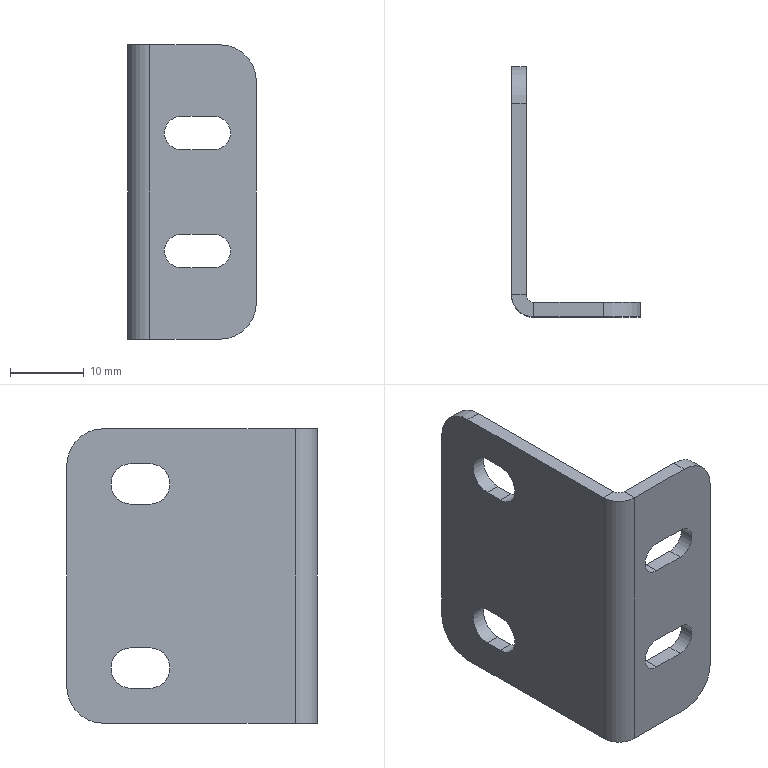Part | SolidWorks | features HoleWzd 2, Fillet 1, FlatPattern 1, SMBaseFlange 1, SheetMetal 1 | 1 solid | 34 faces | box 17.5 x 34 x 40 mm | volume 3554 mm3 | plane 20 | cylinder 14 | commonest cylinder face diameters 4.5 x4 5.5 x4 10 x4 2 x1 6 x1
STEP:
#1=CARTESIAN_POINT('',(0.,-31.,40.));
#2=VERTEX_POINT('',#1);
#3=CARTESIAN_POINT('',(2.,-31.,40.));
#4=VERTEX_POINT('',#3);
#5=CARTESIAN_POINT('',(0.,-31.,40.));
#6=DIRECTION('',(1.,0.,0.));
#7=VECTOR('',#6,1000.);
#8=LINE('',#5,#7);
#9=EDGE_CURVE('',#2,#4,#8,.T.);
#10=ORIENTED_EDGE('',*,*,#9,.F.);
#11=CARTESIAN_POINT('',(3.,-34.,40.));
#12=VERTEX_POINT('',#11);
#13=CARTESIAN_POINT('',(3.,-31.,40.));
#14=DIRECTION('',(0.,0.,1.));
#15=DIRECTION('',(-1.,0.,0.));
#16=AXIS2_PLACEMENT_3D('',#13,#14,#15);
#17=CIRCLE('',#16,3.);
#18=EDGE_CURVE('',#2,#12,#17,.T.);
#19=ORIENTED_EDGE('',*,*,#18,.T.);
#20=CARTESIAN_POINT('',(3.,-32.,40.));
#21=VERTEX_POINT('',#20);
#22=CARTESIAN_POINT('',(3.,-32.,40.));
#23=DIRECTION('',(0.,-1.,0.));
#24=VECTOR('',#23,1000.);
#25=LINE('',#22,#24);
#26=EDGE_CURVE('',#21,#12,#25,.T.);
#27=ORIENTED_EDGE('',*,*,#26,.F.);
#28=CARTESIAN_POINT('',(3.,-31.,40.));
#29=DIRECTION('',(0.,0.,1.));
#30=DIRECTION('',(1.,0.,0.));
#31=AXIS2_PLACEMENT_3D('',#28,#29,#30);
#32=CIRCLE('',#31,1.);
#33=EDGE_CURVE('',#4,#21,#32,.T.);
#34=ORIENTED_EDGE('',*,*,#33,.F.);
#35=EDGE_LOOP('',(#10,#19,#27,#34));
#36=FACE_OUTER_BOUND('',#35,.T.);
#37=CARTESIAN_POINT('',(0.,-31.,40.));
#38=DIRECTION('',(0.,0.,1.));
#39=DIRECTION('',(1.,0.,0.));
#40=AXIS2_PLACEMENT_3D('',#37,#38,#39);
#41=PLANE('',#40);
#42=ADVANCED_FACE('',(#36),#41,.T.);
#43=CARTESIAN_POINT('',(2.,-5.,40.));
#44=VERTEX_POINT('',#43);
#45=CARTESIAN_POINT('',(2.,0.,40.));
#46=DIRECTION('',(0.,-1.,0.));
#47=VECTOR('',#46,1000.);
#48=LINE('',#45,#47);
#49=EDGE_CURVE('',#44,#4,#48,.T.);
#50=ORIENTED_EDGE('',*,*,#49,.F.);
#51=CARTESIAN_POINT('',(0.,-5.,40.));
#52=VERTEX_POINT('',#51);
#53=CARTESIAN_POINT('',(3.,-5.,40.));
#54=DIRECTION('',(-1.,0.,0.));
#55=VECTOR('',#54,1000.);
#56=LINE('',#53,#55);
#57=EDGE_CURVE('',#44,#52,#56,.T.);
#58=ORIENTED_EDGE('',*,*,#57,.T.);
#59=CARTESIAN_POINT('',(0.,0.,40.));
#60=DIRECTION('',(0.,-1.,0.));
#61=VECTOR('',#60,1000.);
#62=LINE('',#59,#61);
#63=EDGE_CURVE('',#52,#2,#62,.T.);
#64=ORIENTED_EDGE('',*,*,#63,.T.);
#65=ORIENTED_EDGE('',*,*,#9,.T.);
#66=EDGE_LOOP('',(#50,#58,#64,#65));
#67=FACE_OUTER_BOUND('',#66,.T.);
#68=CARTESIAN_POINT('',(3.,-32.,40.));
#69=DIRECTION('',(0.,0.,1.));
#70=DIRECTION('',(1.,0.,0.));
#71=AXIS2_PLACEMENT_3D('',#68,#69,#70);
#72=PLANE('',#71);
#73=ADVANCED_FACE('',(#67),#72,.T.);
#74=CARTESIAN_POINT('',(3.,-34.,0.));
#75=VERTEX_POINT('',#74);
#76=CARTESIAN_POINT('',(3.,-32.,0.));
#77=VERTEX_POINT('',#76);
#78=CARTESIAN_POINT('',(3.,-34.,0.));
#79=DIRECTION('',(0.,1.,0.));
#80=VECTOR('',#79,1000.);
#81=LINE('',#78,#80);
#82=EDGE_CURVE('',#75,#77,#81,.T.);
#83=ORIENTED_EDGE('',*,*,#82,.F.);
#84=CARTESIAN_POINT('',(0.,-31.,0.));
#85=VERTEX_POINT('',#84);
#86=CARTESIAN_POINT('',(3.,-31.,0.));
#87=DIRECTION('',(0.,0.,1.));
#88=DIRECTION('',(-1.,0.,0.));
#89=AXIS2_PLACEMENT_3D('',#86,#87,#88);
#90=CIRCLE('',#89,3.);
#91=EDGE_CURVE('',#85,#75,#90,.T.);
#92=ORIENTED_EDGE('',*,*,#91,.F.);
#93=CARTESIAN_POINT('',(2.,-31.,0.));
#94=VERTEX_POINT('',#93);
#95=CARTESIAN_POINT('',(2.,-31.,0.));
#96=DIRECTION('',(-1.,0.,0.));
#97=VECTOR('',#96,1000.);
#98=LINE('',#95,#97);
#99=EDGE_CURVE('',#94,#85,#98,.T.);
#100=ORIENTED_EDGE('',*,*,#99,.F.);
#101=CARTESIAN_POINT('',(3.,-31.,0.));
#102=DIRECTION('',(0.,0.,1.));
#103=DIRECTION('',(1.,0.,0.));
#104=AXIS2_PLACEMENT_3D('',#101,#102,#103);
#105=CIRCLE('',#104,1.);
#106=EDGE_CURVE('',#94,#77,#105,.T.);
#107=ORIENTED_EDGE('',*,*,#106,.T.);
#108=EDGE_LOOP('',(#83,#92,#100,#107));
#109=FACE_OUTER_BOUND('',#108,.T.);
#110=CARTESIAN_POINT('',(3.,-34.,0.));
#111=DIRECTION('',(0.,0.,-1.));
#112=DIRECTION('',(-1.,0.,0.));
#113=AXIS2_PLACEMENT_3D('',#110,#111,#112);
#114=PLANE('',#113);
#115=ADVANCED_FACE('',(#109),#114,.T.);
#116=CARTESIAN_POINT('',(12.5,-32.,0.));
#117=VERTEX_POINT('',#116);
#118=CARTESIAN_POINT('',(0.,-32.,0.));
#119=DIRECTION('',(1.,0.,0.));
#120=VECTOR('',#119,1000.);
#121=LINE('',#118,#120);
#122=EDGE_CURVE('',#77,#117,#121,.T.);
#123=ORIENTED_EDGE('',*,*,#122,.T.);
#124=CARTESIAN_POINT('',(12.5,-34.,0.));
#125=VERTEX_POINT('',#124);
#126=CARTESIAN_POINT('',(12.5,-31.,0.));
#127=DIRECTION('',(0.,-1.,0.));
#128=VECTOR('',#127,1000.);
#129=LINE('',#126,#128);
#130=EDGE_CURVE('',#117,#125,#129,.T.);
#131=ORIENTED_EDGE('',*,*,#130,.T.);
#132=CARTESIAN_POINT('',(0.,-34.,0.));
#133=DIRECTION('',(1.,0.,0.));
#134=VECTOR('',#133,1000.);
#135=LINE('',#132,#134);
#136=EDGE_CURVE('',#75,#125,#135,.T.);
#137=ORIENTED_EDGE('',*,*,#136,.F.);
#138=ORIENTED_EDGE('',*,*,#82,.T.);
#139=EDGE_LOOP('',(#123,#131,#137,#138));
#140=FACE_OUTER_BOUND('',#139,.T.);
#141=CARTESIAN_POINT('',(2.,-31.,0.));
#142=DIRECTION('',(0.,0.,-1.));
#143=DIRECTION('',(-1.,0.,0.));
#144=AXIS2_PLACEMENT_3D('',#141,#142,#143);
#145=PLANE('',#144);
#146=ADVANCED_FACE('',(#140),#145,.T.);
#147=CARTESIAN_POINT('',(11.75,-34.,9.75));
#148=VERTEX_POINT('',#147);
#149=CARTESIAN_POINT('',(7.25,-34.,9.75));
#150=VERTEX_POINT('',#149);
#151=CARTESIAN_POINT('',(0.,-34.,9.75));
#152=DIRECTION('',(-1.,0.,0.));
#153=VECTOR('',#152,1000.);
#154=LINE('',#151,#153);
#155=EDGE_CURVE('',#148,#150,#154,.T.);
#156=ORIENTED_EDGE('',*,*,#155,.T.);
#157=CARTESIAN_POINT('',(7.25,-34.,14.25));
#158=VERTEX_POINT('',#157);
#159=CARTESIAN_POINT('',(7.25,-34.,12.));
#160=DIRECTION('',(0.,1.,0.));
#161=DIRECTION('',(0.,0.,1.));
#162=AXIS2_PLACEMENT_3D('',#159,#160,#161);
#163=CIRCLE('',#162,2.25);
#164=EDGE_CURVE('',#150,#158,#163,.T.);
#165=ORIENTED_EDGE('',*,*,#164,.T.);
#166=CARTESIAN_POINT('',(11.75,-34.,14.25));
#167=VERTEX_POINT('',#166);
#168=CARTESIAN_POINT('',(0.,-34.,14.25));
#169=DIRECTION('',(1.,0.,0.));
#170=VECTOR('',#169,1000.);
#171=LINE('',#168,#170);
#172=EDGE_CURVE('',#158,#167,#171,.T.);
#173=ORIENTED_EDGE('',*,*,#172,.T.);
#174=CARTESIAN_POINT('',(11.75,-34.,12.));
#175=DIRECTION('',(0.,1.,0.));
#176=DIRECTION('',(0.,0.,1.));
#177=AXIS2_PLACEMENT_3D('',#174,#175,#176);
#178=CIRCLE('',#177,2.25);
#179=EDGE_CURVE('',#167,#148,#178,.T.);
#180=ORIENTED_EDGE('',*,*,#179,.T.);
#181=EDGE_LOOP('',(#156,#165,#173,#180));
#182=FACE_BOUND('',#181,.T.);
#183=CARTESIAN_POINT('',(7.25,-34.,30.25));
#184=VERTEX_POINT('',#183);
#185=CARTESIAN_POINT('',(11.75,-34.,30.25));
#186=VERTEX_POINT('',#185);
#187=CARTESIAN_POINT('',(0.,-34.,30.25));
#188=DIRECTION('',(1.,0.,0.));
#189=VECTOR('',#188,1000.);
#190=LINE('',#187,#189);
#191=EDGE_CURVE('',#184,#186,#190,.T.);
#192=ORIENTED_EDGE('',*,*,#191,.T.);
#193=CARTESIAN_POINT('',(11.75,-34.,25.75));
#194=VERTEX_POINT('',#193);
#195=CARTESIAN_POINT('',(11.75,-34.,28.));
#196=DIRECTION('',(0.,1.,0.));
#197=DIRECTION('',(0.,0.,1.));
#198=AXIS2_PLACEMENT_3D('',#195,#196,#197);
#199=CIRCLE('',#198,2.25);
#200=EDGE_CURVE('',#186,#194,#199,.T.);
#201=ORIENTED_EDGE('',*,*,#200,.T.);
#202=CARTESIAN_POINT('',(7.25,-34.,25.75));
#203=VERTEX_POINT('',#202);
#204=CARTESIAN_POINT('',(0.,-34.,25.75));
#205=DIRECTION('',(-1.,0.,0.));
#206=VECTOR('',#205,1000.);
#207=LINE('',#204,#206);
#208=EDGE_CURVE('',#194,#203,#207,.T.);
#209=ORIENTED_EDGE('',*,*,#208,.T.);
#210=CARTESIAN_POINT('',(7.25,-34.,28.));
#211=DIRECTION('',(0.,1.,0.));
#212=DIRECTION('',(0.,0.,1.));
#213=AXIS2_PLACEMENT_3D('',#210,#211,#212);
#214=CIRCLE('',#213,2.25);
#215=EDGE_CURVE('',#203,#184,#214,.T.);
#216=ORIENTED_EDGE('',*,*,#215,.T.);
#217=EDGE_LOOP('',(#192,#201,#209,#216));
#218=FACE_BOUND('',#217,.T.);
#219=ORIENTED_EDGE('',*,*,#136,.T.);
#220=CARTESIAN_POINT('',(17.5,-34.,5.));
#221=VERTEX_POINT('',#220);
#222=CARTESIAN_POINT('',(12.5,-34.,5.));
#223=DIRECTION('',(0.,-1.,0.));
#224=DIRECTION('',(0.,0.,1.));
#225=AXIS2_PLACEMENT_3D('',#222,#223,#224);
#226=CIRCLE('',#225,5.);
#227=EDGE_CURVE('',#125,#221,#226,.T.);
#228=ORIENTED_EDGE('',*,*,#227,.T.);
#229=CARTESIAN_POINT('',(17.5,-34.,35.));
#230=VERTEX_POINT('',#229);
#231=CARTESIAN_POINT('',(17.5,-34.,40.));
#232=DIRECTION('',(0.,0.,-1.));
#233=VECTOR('',#232,1000.);
#234=LINE('',#231,#233);
#235=EDGE_CURVE('',#230,#221,#234,.T.);
#236=ORIENTED_EDGE('',*,*,#235,.F.);
#237=CARTESIAN_POINT('',(12.5,-34.,40.));
#238=VERTEX_POINT('',#237);
#239=CARTESIAN_POINT('',(12.5,-34.,35.));
#240=DIRECTION('',(0.,-1.,0.));
#241=DIRECTION('',(0.,0.,1.));
#242=AXIS2_PLACEMENT_3D('',#239,#240,#241);
#243=CIRCLE('',#242,5.);
#244=EDGE_CURVE('',#230,#238,#243,.T.);
#245=ORIENTED_EDGE('',*,*,#244,.T.);
#246=CARTESIAN_POINT('',(0.,-34.,40.));
#247=DIRECTION('',(1.,0.,0.));
#248=VECTOR('',#247,1000.);
#249=LINE('',#246,#248);
#250=EDGE_CURVE('',#12,#238,#249,.T.);
#251=ORIENTED_EDGE('',*,*,#250,.F.);
#252=CARTESIAN_POINT('',(3.,-34.,40.));
#253=DIRECTION('',(0.,0.,-1.));
#254=VECTOR('',#253,1000.);
#255=LINE('',#252,#254);
#256=EDGE_CURVE('',#12,#75,#255,.T.);
#257=ORIENTED_EDGE('',*,*,#256,.T.);
#258=EDGE_LOOP('',(#219,#228,#236,#245,#251,#257));
#259=FACE_OUTER_BOUND('',#258,.T.);
#260=CARTESIAN_POINT('',(0.,-34.,40.));
#261=DIRECTION('',(0.,1.,0.));
#262=DIRECTION('',(0.,0.,1.));
#263=AXIS2_PLACEMENT_3D('',#260,#261,#262);
#264=PLANE('',#263);
#265=ADVANCED_FACE('',(#182,#218,#259),#264,.F.);
#266=ORIENTED_EDGE('',*,*,#235,.T.);
#267=CARTESIAN_POINT('',(17.5,-32.,5.));
#268=VERTEX_POINT('',#267);
#269=CARTESIAN_POINT('',(17.5,-32.,5.));
#270=DIRECTION('',(0.,1.,0.));
#271=VECTOR('',#270,1000.);
#272=LINE('',#269,#271);
#273=EDGE_CURVE('',#221,#268,#272,.T.);
#274=ORIENTED_EDGE('',*,*,#273,.T.);
#275=CARTESIAN_POINT('',(17.5,-32.,35.));
#276=VERTEX_POINT('',#275);
#277=CARTESIAN_POINT('',(17.5,-32.,40.));
#278=DIRECTION('',(0.,0.,-1.));
#279=VECTOR('',#278,1000.);
#280=LINE('',#277,#279);
#281=EDGE_CURVE('',#276,#268,#280,.T.);
#282=ORIENTED_EDGE('',*,*,#281,.F.);
#283=CARTESIAN_POINT('',(17.5,-32.,35.));
#284=DIRECTION('',(0.,-1.,0.));
#285=VECTOR('',#284,1000.);
#286=LINE('',#283,#285);
#287=EDGE_CURVE('',#276,#230,#286,.T.);
#288=ORIENTED_EDGE('',*,*,#287,.T.);
#289=EDGE_LOOP('',(#266,#274,#282,#288));
#290=FACE_OUTER_BOUND('',#289,.T.);
#291=CARTESIAN_POINT('',(17.5,-32.,40.));
#292=DIRECTION('',(1.,0.,0.));
#293=DIRECTION('',(0.,0.,-1.));
#294=AXIS2_PLACEMENT_3D('',#291,#292,#293);
#295=PLANE('',#294);
#296=ADVANCED_FACE('',(#290),#295,.T.);
#297=CARTESIAN_POINT('',(11.75,-32.,14.25));
#298=VERTEX_POINT('',#297);
#299=CARTESIAN_POINT('',(11.75,-32.,9.75));
#300=VERTEX_POINT('',#299);
#301=CARTESIAN_POINT('',(11.75,-32.,12.));
#302=DIRECTION('',(0.,1.,0.));
#303=DIRECTION('',(0.,0.,1.));
#304=AXIS2_PLACEMENT_3D('',#301,#302,#303);
#305=CIRCLE('',#304,2.25);
#306=EDGE_CURVE('',#298,#300,#305,.T.);
#307=ORIENTED_EDGE('',*,*,#306,.F.);
#308=CARTESIAN_POINT('',(7.25,-32.,14.25));
#309=VERTEX_POINT('',#308);
#310=CARTESIAN_POINT('',(7.25,-32.,14.25));
#311=DIRECTION('',(1.,0.,0.));
#312=VECTOR('',#311,1000.);
#313=LINE('',#310,#312);
#314=EDGE_CURVE('',#309,#298,#313,.T.);
#315=ORIENTED_EDGE('',*,*,#314,.F.);
#316=CARTESIAN_POINT('',(7.25,-32.,9.75));
#317=VERTEX_POINT('',#316);
#318=CARTESIAN_POINT('',(7.25,-32.,12.));
#319=DIRECTION('',(0.,1.,0.));
#320=DIRECTION('',(0.,0.,1.));
#321=AXIS2_PLACEMENT_3D('',#318,#319,#320);
#322=CIRCLE('',#321,2.25);
#323=EDGE_CURVE('',#317,#309,#322,.T.);
#324=ORIENTED_EDGE('',*,*,#323,.F.);
#325=CARTESIAN_POINT('',(7.25,-32.,9.75));
#326=DIRECTION('',(1.,0.,0.));
#327=VECTOR('',#326,1000.);
#328=LINE('',#325,#327);
#329=EDGE_CURVE('',#317,#300,#328,.T.);
#330=ORIENTED_EDGE('',*,*,#329,.T.);
#331=EDGE_LOOP('',(#307,#315,#324,#330));
#332=FACE_BOUND('',#331,.T.);
#333=CARTESIAN_POINT('',(11.75,-32.,30.25));
#334=VERTEX_POINT('',#333);
#335=CARTESIAN_POINT('',(11.75,-32.,25.75));
#336=VERTEX_POINT('',#335);
#337=CARTESIAN_POINT('',(11.75,-32.,28.));
#338=DIRECTION('',(0.,1.,0.));
#339=DIRECTION('',(0.,0.,1.));
#340=AXIS2_PLACEMENT_3D('',#337,#338,#339);
#341=CIRCLE('',#340,2.25);
#342=EDGE_CURVE('',#334,#336,#341,.T.);
#343=ORIENTED_EDGE('',*,*,#342,.F.);
#344=CARTESIAN_POINT('',(7.25,-32.,30.25));
#345=VERTEX_POINT('',#344);
#346=CARTESIAN_POINT('',(7.25,-32.,30.25));
#347=DIRECTION('',(1.,0.,0.));
#348=VECTOR('',#347,1000.);
#349=LINE('',#346,#348);
#350=EDGE_CURVE('',#345,#334,#349,.T.);
#351=ORIENTED_EDGE('',*,*,#350,.F.);
#352=CARTESIAN_POINT('',(7.25,-32.,25.75));
#353=VERTEX_POINT('',#352);
#354=CARTESIAN_POINT('',(7.25,-32.,28.));
#355=DIRECTION('',(0.,1.,0.));
#356=DIRECTION('',(0.,0.,1.));
#357=AXIS2_PLACEMENT_3D('',#354,#355,#356);
#358=CIRCLE('',#357,2.25);
#359=EDGE_CURVE('',#353,#345,#358,.T.);
#360=ORIENTED_EDGE('',*,*,#359,.F.);
#361=CARTESIAN_POINT('',(7.25,-32.,25.75));
#362=DIRECTION('',(1.,0.,0.));
#363=VECTOR('',#362,1000.);
#364=LINE('',#361,#363);
#365=EDGE_CURVE('',#353,#336,#364,.T.);
#366=ORIENTED_EDGE('',*,*,#365,.T.);
#367=EDGE_LOOP('',(#343,#351,#360,#366));
#368=FACE_BOUND('',#367,.T.);
#369=ORIENTED_EDGE('',*,*,#281,.T.);
#370=CARTESIAN_POINT('',(12.5,-32.,5.));
#371=DIRECTION('',(0.,1.,0.));
#372=DIRECTION('',(0.,0.,1.));
#373=AXIS2_PLACEMENT_3D('',#370,#371,#372);
#374=CIRCLE('',#373,5.);
#375=EDGE_CURVE('',#268,#117,#374,.T.);
#376=ORIENTED_EDGE('',*,*,#375,.T.);
#377=ORIENTED_EDGE('',*,*,#122,.F.);
#378=CARTESIAN_POINT('',(3.,-32.,40.));
#379=DIRECTION('',(0.,0.,-1.));
#380=VECTOR('',#379,1000.);
#381=LINE('',#378,#380);
#382=EDGE_CURVE('',#21,#77,#381,.T.);
#383=ORIENTED_EDGE('',*,*,#382,.F.);
#384=CARTESIAN_POINT('',(12.5,-32.,40.));
#385=VERTEX_POINT('',#384);
#386=CARTESIAN_POINT('',(0.,-32.,40.));
#387=DIRECTION('',(1.,0.,0.));
#388=VECTOR('',#387,1000.);
#389=LINE('',#386,#388);
#390=EDGE_CURVE('',#21,#385,#389,.T.);
#391=ORIENTED_EDGE('',*,*,#390,.T.);
#392=CARTESIAN_POINT('',(12.5,-32.,35.));
#393=DIRECTION('',(0.,1.,0.));
#394=DIRECTION('',(0.,0.,1.));
#395=AXIS2_PLACEMENT_3D('',#392,#393,#394);
#396=CIRCLE('',#395,5.);
#397=EDGE_CURVE('',#385,#276,#396,.T.);
#398=ORIENTED_EDGE('',*,*,#397,.T.);
#399=EDGE_LOOP('',(#369,#376,#377,#383,#391,#398));
#400=FACE_OUTER_BOUND('',#399,.T.);
#401=CARTESIAN_POINT('',(0.,-32.,40.));
#402=DIRECTION('',(0.,1.,0.));
#403=DIRECTION('',(0.,0.,1.));
#404=AXIS2_PLACEMENT_3D('',#401,#402,#403);
#405=PLANE('',#404);
#406=ADVANCED_FACE('',(#332,#368,#400),#405,.T.);
#407=ORIENTED_EDGE('',*,*,#106,.F.);
#408=CARTESIAN_POINT('',(2.,-31.,40.));
#409=DIRECTION('',(0.,0.,-1.));
#410=VECTOR('',#409,1000.);
#411=LINE('',#408,#410);
#412=EDGE_CURVE('',#4,#94,#411,.T.);
#413=ORIENTED_EDGE('',*,*,#412,.F.);
#414=ORIENTED_EDGE('',*,*,#33,.T.);
#415=ORIENTED_EDGE('',*,*,#382,.T.);
#416=EDGE_LOOP('',(#407,#413,#414,#415));
#417=FACE_OUTER_BOUND('',#416,.T.);
#418=CARTESIAN_POINT('',(3.,-31.,40.));
#419=DIRECTION('',(0.,0.,-1.));
#420=DIRECTION('',(-1.,0.,0.));
#421=AXIS2_PLACEMENT_3D('',#418,#419,#420);
#422=CYLINDRICAL_SURFACE('',#421,1.);
#423=ADVANCED_FACE('',(#417),#422,.F.);
#424=CARTESIAN_POINT('',(2.,-8.75,4.75));
#425=VERTEX_POINT('',#424);
#426=CARTESIAN_POINT('',(2.,-8.75,10.25));
#427=VERTEX_POINT('',#426);
#428=CARTESIAN_POINT('',(2.,-8.75,7.5));
#429=DIRECTION('',(1.,0.,0.));
#430=DIRECTION('',(0.,0.,-1.));
#431=AXIS2_PLACEMENT_3D('',#428,#429,#430);
#432=CIRCLE('',#431,2.75);
#433=EDGE_CURVE('',#425,#427,#432,.T.);
#434=ORIENTED_EDGE('',*,*,#433,.F.);
#435=CARTESIAN_POINT('',(2.,-11.25,4.75));
#436=VERTEX_POINT('',#435);
#437=CARTESIAN_POINT('',(2.,-11.25,4.75));
#438=DIRECTION('',(0.,1.,0.));
#439=VECTOR('',#438,1000.);
#440=LINE('',#437,#439);
#441=EDGE_CURVE('',#436,#425,#440,.T.);
#442=ORIENTED_EDGE('',*,*,#441,.F.);
#443=CARTESIAN_POINT('',(2.,-11.25,10.25));
#444=VERTEX_POINT('',#443);
#445=CARTESIAN_POINT('',(2.,-11.25,7.5));
#446=DIRECTION('',(1.,0.,0.));
#447=DIRECTION('',(0.,0.,-1.));
#448=AXIS2_PLACEMENT_3D('',#445,#446,#447);
#449=CIRCLE('',#448,2.75);
#450=EDGE_CURVE('',#444,#436,#449,.T.);
#451=ORIENTED_EDGE('',*,*,#450,.F.);
#452=CARTESIAN_POINT('',(2.,-11.25,10.25));
#453=DIRECTION('',(0.,1.,0.));
#454=VECTOR('',#453,1000.);
#455=LINE('',#452,#454);
#456=EDGE_CURVE('',#444,#427,#455,.T.);
#457=ORIENTED_EDGE('',*,*,#456,.T.);
#458=EDGE_LOOP('',(#434,#442,#451,#457));
#459=FACE_BOUND('',#458,.T.);
#460=CARTESIAN_POINT('',(2.,-11.25,35.25));
#461=VERTEX_POINT('',#460);
#462=CARTESIAN_POINT('',(2.,-11.25,29.75));
#463=VERTEX_POINT('',#462);
#464=CARTESIAN_POINT('',(2.,-11.25,32.5));
#465=DIRECTION('',(1.,0.,0.));
#466=DIRECTION('',(0.,0.,-1.));
#467=AXIS2_PLACEMENT_3D('',#464,#465,#466);
#468=CIRCLE('',#467,2.75);
#469=EDGE_CURVE('',#461,#463,#468,.T.);
#470=ORIENTED_EDGE('',*,*,#469,.F.);
#471=CARTESIAN_POINT('',(2.,-8.75,35.25));
#472=VERTEX_POINT('',#471);
#473=CARTESIAN_POINT('',(2.,-11.25,35.25));
#474=DIRECTION('',(0.,1.,0.));
#475=VECTOR('',#474,1000.);
#476=LINE('',#473,#475);
#477=EDGE_CURVE('',#461,#472,#476,.T.);
#478=ORIENTED_EDGE('',*,*,#477,.T.);
#479=CARTESIAN_POINT('',(2.,-8.75,29.75));
#480=VERTEX_POINT('',#479);
#481=CARTESIAN_POINT('',(2.,-8.75,32.5));
#482=DIRECTION('',(1.,0.,0.));
#483=DIRECTION('',(0.,0.,-1.));
#484=AXIS2_PLACEMENT_3D('',#481,#482,#483);
#485=CIRCLE('',#484,2.75);
#486=EDGE_CURVE('',#480,#472,#485,.T.);
#487=ORIENTED_EDGE('',*,*,#486,.F.);
#488=CARTESIAN_POINT('',(2.,-11.25,29.75));
#489=DIRECTION('',(0.,1.,0.));
#490=VECTOR('',#489,1000.);
#491=LINE('',#488,#490);
#492=EDGE_CURVE('',#463,#480,#491,.T.);
#493=ORIENTED_EDGE('',*,*,#492,.F.);
#494=EDGE_LOOP('',(#470,#478,#487,#493));
#495=FACE_BOUND('',#494,.T.);
#496=CARTESIAN_POINT('',(2.,0.,35.));
#497=VERTEX_POINT('',#496);
#498=CARTESIAN_POINT('',(2.,0.,5.));
#499=VERTEX_POINT('',#498);
#500=CARTESIAN_POINT('',(2.,0.,40.));
#501=DIRECTION('',(0.,0.,-1.));
#502=VECTOR('',#501,1000.);
#503=LINE('',#500,#502);
#504=EDGE_CURVE('',#497,#499,#503,.T.);
#505=ORIENTED_EDGE('',*,*,#504,.F.);
#506=CARTESIAN_POINT('',(2.,-5.,35.));
#507=DIRECTION('',(1.,0.,0.));
#508=DIRECTION('',(0.,1.,0.));
#509=AXIS2_PLACEMENT_3D('',#506,#507,#508);
#510=CIRCLE('',#509,5.);
#511=EDGE_CURVE('',#497,#44,#510,.T.);
#512=ORIENTED_EDGE('',*,*,#511,.T.);
#513=ORIENTED_EDGE('',*,*,#49,.T.);
#514=ORIENTED_EDGE('',*,*,#412,.T.);
#515=CARTESIAN_POINT('',(2.,-5.,0.));
#516=VERTEX_POINT('',#515);
#517=CARTESIAN_POINT('',(2.,0.,0.));
#518=DIRECTION('',(0.,-1.,0.));
#519=VECTOR('',#518,1000.);
#520=LINE('',#517,#519);
#521=EDGE_CURVE('',#516,#94,#520,.T.);
#522=ORIENTED_EDGE('',*,*,#521,.F.);
#523=CARTESIAN_POINT('',(2.,-5.,5.));
#524=DIRECTION('',(1.,0.,0.));
#525=DIRECTION('',(0.,1.,0.));
#526=AXIS2_PLACEMENT_3D('',#523,#524,#525);
#527=CIRCLE('',#526,5.);
#528=EDGE_CURVE('',#516,#499,#527,.T.);
#529=ORIENTED_EDGE('',*,*,#528,.T.);
#530=EDGE_LOOP('',(#505,#512,#513,#514,#522,#529));
#531=FACE_OUTER_BOUND('',#530,.T.);
#532=CARTESIAN_POINT('',(2.,0.,40.));
#533=DIRECTION('',(1.,0.,0.));
#534=DIRECTION('',(0.,1.,0.));
#535=AXIS2_PLACEMENT_3D('',#532,#533,#534);
#536=PLANE('',#535);
#537=ADVANCED_FACE('',(#459,#495,#531),#536,.T.);
#538=CARTESIAN_POINT('',(0.,0.,35.));
#539=VERTEX_POINT('',#538);
#540=CARTESIAN_POINT('',(0.,0.,5.));
#541=VERTEX_POINT('',#540);
#542=CARTESIAN_POINT('',(0.,0.,40.));
#543=DIRECTION('',(0.,0.,-1.));
#544=VECTOR('',#543,1000.);
#545=LINE('',#542,#544);
#546=EDGE_CURVE('',#539,#541,#545,.T.);
#547=ORIENTED_EDGE('',*,*,#546,.F.);
#548=CARTESIAN_POINT('',(0.,0.,35.));
#549=DIRECTION('',(1.,0.,0.));
#550=VECTOR('',#549,1000.);
#551=LINE('',#548,#550);
#552=EDGE_CURVE('',#539,#497,#551,.T.);
#553=ORIENTED_EDGE('',*,*,#552,.T.);
#554=ORIENTED_EDGE('',*,*,#504,.T.);
#555=CARTESIAN_POINT('',(0.,0.,5.));
#556=DIRECTION('',(-1.,0.,0.));
#557=VECTOR('',#556,1000.);
#558=LINE('',#555,#557);
#559=EDGE_CURVE('',#499,#541,#558,.T.);
#560=ORIENTED_EDGE('',*,*,#559,.T.);
#561=EDGE_LOOP('',(#547,#553,#554,#560));
#562=FACE_OUTER_BOUND('',#561,.T.);
#563=CARTESIAN_POINT('',(0.,0.,40.));
#564=DIRECTION('',(0.,1.,0.));
#565=DIRECTION('',(-1.,0.,0.));
#566=AXIS2_PLACEMENT_3D('',#563,#564,#565);
#567=PLANE('',#566);
#568=ADVANCED_FACE('',(#562),#567,.T.);
#569=CARTESIAN_POINT('',(0.,-11.25,10.25));
#570=VERTEX_POINT('',#569);
#571=CARTESIAN_POINT('',(0.,-11.25,4.75));
#572=VERTEX_POINT('',#571);
#573=CARTESIAN_POINT('',(0.,-11.25,7.5));
#574=DIRECTION('',(1.,0.,0.));
#575=DIRECTION('',(0.,1.,0.));
#576=AXIS2_PLACEMENT_3D('',#573,#574,#575);
#577=CIRCLE('',#576,2.75);
#578=EDGE_CURVE('',#570,#572,#577,.T.);
#579=ORIENTED_EDGE('',*,*,#578,.T.);
#580=CARTESIAN_POINT('',(0.,-8.75,4.75));
#581=VERTEX_POINT('',#580);
#582=CARTESIAN_POINT('',(0.,0.,4.75));
#583=DIRECTION('',(0.,1.,0.));
#584=VECTOR('',#583,1000.);
#585=LINE('',#582,#584);
#586=EDGE_CURVE('',#572,#581,#585,.T.);
#587=ORIENTED_EDGE('',*,*,#586,.T.);
#588=CARTESIAN_POINT('',(0.,-8.75,10.25));
#589=VERTEX_POINT('',#588);
#590=CARTESIAN_POINT('',(0.,-8.75,7.5));
#591=DIRECTION('',(1.,0.,0.));
#592=DIRECTION('',(0.,1.,0.));
#593=AXIS2_PLACEMENT_3D('',#590,#591,#592);
#594=CIRCLE('',#593,2.75);
#595=EDGE_CURVE('',#581,#589,#594,.T.);
#596=ORIENTED_EDGE('',*,*,#595,.T.);
#597=CARTESIAN_POINT('',(0.,0.,10.25));
#598=DIRECTION('',(0.,-1.,0.));
#599=VECTOR('',#598,1000.);
#600=LINE('',#597,#599);
#601=EDGE_CURVE('',#589,#570,#600,.T.);
#602=ORIENTED_EDGE('',*,*,#601,.T.);
#603=EDGE_LOOP('',(#579,#587,#596,#602));
#604=FACE_BOUND('',#603,.T.);
#605=CARTESIAN_POINT('',(0.,-8.75,35.25));
#606=VERTEX_POINT('',#605);
#607=CARTESIAN_POINT('',(0.,-11.25,35.25));
#608=VERTEX_POINT('',#607);
#609=CARTESIAN_POINT('',(0.,0.,35.25));
#610=DIRECTION('',(0.,-1.,0.));
#611=VECTOR('',#610,1000.);
#612=LINE('',#609,#611);
#613=EDGE_CURVE('',#606,#608,#612,.T.);
#614=ORIENTED_EDGE('',*,*,#613,.T.);
#615=CARTESIAN_POINT('',(0.,-11.25,29.75));
#616=VERTEX_POINT('',#615);
#617=CARTESIAN_POINT('',(0.,-11.25,32.5));
#618=DIRECTION('',(1.,0.,0.));
#619=DIRECTION('',(0.,1.,0.));
#620=AXIS2_PLACEMENT_3D('',#617,#618,#619);
#621=CIRCLE('',#620,2.75);
#622=EDGE_CURVE('',#608,#616,#621,.T.);
#623=ORIENTED_EDGE('',*,*,#622,.T.);
#624=CARTESIAN_POINT('',(0.,-8.75,29.75));
#625=VERTEX_POINT('',#624);
#626=CARTESIAN_POINT('',(0.,0.,29.75));
#627=DIRECTION('',(0.,1.,0.));
#628=VECTOR('',#627,1000.);
#629=LINE('',#626,#628);
#630=EDGE_CURVE('',#616,#625,#629,.T.);
#631=ORIENTED_EDGE('',*,*,#630,.T.);
#632=CARTESIAN_POINT('',(0.,-8.75,32.5));
#633=DIRECTION('',(1.,0.,0.));
#634=DIRECTION('',(0.,1.,0.));
#635=AXIS2_PLACEMENT_3D('',#632,#633,#634);
#636=CIRCLE('',#635,2.75);
#637=EDGE_CURVE('',#625,#606,#636,.T.);
#638=ORIENTED_EDGE('',*,*,#637,.T.);
#639=EDGE_LOOP('',(#614,#623,#631,#638));
#640=FACE_BOUND('',#639,.T.);
#641=ORIENTED_EDGE('',*,*,#63,.F.);
#642=CARTESIAN_POINT('',(0.,-5.,35.));
#643=DIRECTION('',(-1.,0.,0.));
#644=DIRECTION('',(0.,1.,0.));
#645=AXIS2_PLACEMENT_3D('',#642,#643,#644);
#646=CIRCLE('',#645,5.);
#647=EDGE_CURVE('',#52,#539,#646,.T.);
#648=ORIENTED_EDGE('',*,*,#647,.T.);
#649=ORIENTED_EDGE('',*,*,#546,.T.);
#650=CARTESIAN_POINT('',(0.,-5.,0.));
#651=VERTEX_POINT('',#650);
#652=CARTESIAN_POINT('',(0.,-5.,5.));
#653=DIRECTION('',(-1.,0.,0.));
#654=DIRECTION('',(0.,1.,0.));
#655=AXIS2_PLACEMENT_3D('',#652,#653,#654);
#656=CIRCLE('',#655,5.);
#657=EDGE_CURVE('',#541,#651,#656,.T.);
#658=ORIENTED_EDGE('',*,*,#657,.T.);
#659=CARTESIAN_POINT('',(0.,0.,0.));
#660=DIRECTION('',(0.,-1.,0.));
#661=VECTOR('',#660,1000.);
#662=LINE('',#659,#661);
#663=EDGE_CURVE('',#651,#85,#662,.T.);
#664=ORIENTED_EDGE('',*,*,#663,.T.);
#665=CARTESIAN_POINT('',(0.,-31.,40.));
#666=DIRECTION('',(0.,0.,-1.));
#667=VECTOR('',#666,1000.);
#668=LINE('',#665,#667);
#669=EDGE_CURVE('',#2,#85,#668,.T.);
#670=ORIENTED_EDGE('',*,*,#669,.F.);
#671=EDGE_LOOP('',(#641,#648,#649,#658,#664,#670));
#672=FACE_OUTER_BOUND('',#671,.T.);
#673=CARTESIAN_POINT('',(0.,0.,40.));
#674=DIRECTION('',(1.,0.,0.));
#675=DIRECTION('',(0.,1.,0.));
#676=AXIS2_PLACEMENT_3D('',#673,#674,#675);
#677=PLANE('',#676);
#678=ADVANCED_FACE('',(#604,#640,#672),#677,.F.);
#679=ORIENTED_EDGE('',*,*,#91,.T.);
#680=ORIENTED_EDGE('',*,*,#256,.F.);
#681=ORIENTED_EDGE('',*,*,#18,.F.);
#682=ORIENTED_EDGE('',*,*,#669,.T.);
#683=EDGE_LOOP('',(#679,#680,#681,#682));
#684=FACE_OUTER_BOUND('',#683,.T.);
#685=CARTESIAN_POINT('',(3.,-31.,40.));
#686=DIRECTION('',(0.,0.,-1.));
#687=DIRECTION('',(-1.,0.,0.));
#688=AXIS2_PLACEMENT_3D('',#685,#686,#687);
#689=CYLINDRICAL_SURFACE('',#688,3.);
#690=ADVANCED_FACE('',(#684),#689,.T.);
#691=ORIENTED_EDGE('',*,*,#250,.T.);
#692=CARTESIAN_POINT('',(12.5,-31.,40.));
#693=DIRECTION('',(0.,1.,0.));
#694=VECTOR('',#693,1000.);
#695=LINE('',#692,#694);
#696=EDGE_CURVE('',#238,#385,#695,.T.);
#697=ORIENTED_EDGE('',*,*,#696,.T.);
#698=ORIENTED_EDGE('',*,*,#390,.F.);
#699=ORIENTED_EDGE('',*,*,#26,.T.);
#700=EDGE_LOOP('',(#691,#697,#698,#699));
#701=FACE_OUTER_BOUND('',#700,.T.);
#702=CARTESIAN_POINT('',(3.,-31.,40.));
#703=DIRECTION('',(0.,0.,1.));
#704=DIRECTION('',(1.,0.,0.));
#705=AXIS2_PLACEMENT_3D('',#702,#703,#704);
#706=PLANE('',#705);
#707=ADVANCED_FACE('',(#701),#706,.T.);
#708=ORIENTED_EDGE('',*,*,#663,.F.);
#709=CARTESIAN_POINT('',(2.,-5.,0.));
#710=DIRECTION('',(1.,0.,0.));
#711=VECTOR('',#710,1000.);
#712=LINE('',#709,#711);
#713=EDGE_CURVE('',#651,#516,#712,.T.);
#714=ORIENTED_EDGE('',*,*,#713,.T.);
#715=ORIENTED_EDGE('',*,*,#521,.T.);
#716=ORIENTED_EDGE('',*,*,#99,.T.);
#717=EDGE_LOOP('',(#708,#714,#715,#716));
#718=FACE_OUTER_BOUND('',#717,.T.);
#719=CARTESIAN_POINT('',(3.,-31.,0.));
#720=DIRECTION('',(0.,0.,1.));
#721=DIRECTION('',(1.,0.,0.));
#722=AXIS2_PLACEMENT_3D('',#719,#720,#721);
#723=PLANE('',#722);
#724=ADVANCED_FACE('',(#718),#723,.F.);
#725=CARTESIAN_POINT('',(11.75,-32.,30.25));
#726=DIRECTION('',(0.,-1.,0.));
#727=VECTOR('',#726,1000.);
#728=LINE('',#725,#727);
#729=EDGE_CURVE('',#334,#186,#728,.T.);
#730=ORIENTED_EDGE('',*,*,#729,.F.);
#731=ORIENTED_EDGE('',*,*,#342,.T.);
#732=CARTESIAN_POINT('',(11.75,-32.,25.75));
#733=DIRECTION('',(0.,1.,0.));
#734=VECTOR('',#733,1000.);
#735=LINE('',#732,#734);
#736=EDGE_CURVE('',#194,#336,#735,.T.);
#737=ORIENTED_EDGE('',*,*,#736,.F.);
#738=ORIENTED_EDGE('',*,*,#200,.F.);
#739=EDGE_LOOP('',(#730,#731,#737,#738));
#740=FACE_OUTER_BOUND('',#739,.T.);
#741=CARTESIAN_POINT('',(11.75,-32.,28.));
#742=DIRECTION('',(0.,1.,0.));
#743=DIRECTION('',(0.,0.,1.));
#744=AXIS2_PLACEMENT_3D('',#741,#742,#743);
#745=CYLINDRICAL_SURFACE('',#744,2.25);
#746=ADVANCED_FACE('',(#740),#745,.F.);
#747=CARTESIAN_POINT('',(7.25,-32.,30.25));
#748=DIRECTION('',(0.,1.,0.));
#749=VECTOR('',#748,1000.);
#750=LINE('',#747,#749);
#751=EDGE_CURVE('',#184,#345,#750,.T.);
#752=ORIENTED_EDGE('',*,*,#751,.T.);
#753=ORIENTED_EDGE('',*,*,#350,.T.);
#754=ORIENTED_EDGE('',*,*,#729,.T.);
#755=ORIENTED_EDGE('',*,*,#191,.F.);
#756=EDGE_LOOP('',(#752,#753,#754,#755));
#757=FACE_OUTER_BOUND('',#756,.T.);
#758=CARTESIAN_POINT('',(7.25,-32.,30.25));
#759=DIRECTION('',(0.,0.,1.));
#760=DIRECTION('',(1.,0.,0.));
#761=AXIS2_PLACEMENT_3D('',#758,#759,#760);
#762=PLANE('',#761);
#763=ADVANCED_FACE('',(#757),#762,.F.);
#764=ORIENTED_EDGE('',*,*,#736,.T.);
#765=ORIENTED_EDGE('',*,*,#365,.F.);
#766=CARTESIAN_POINT('',(7.25,-32.,25.75));
#767=DIRECTION('',(0.,-1.,0.));
#768=VECTOR('',#767,1000.);
#769=LINE('',#766,#768);
#770=EDGE_CURVE('',#353,#203,#769,.T.);
#771=ORIENTED_EDGE('',*,*,#770,.T.);
#772=ORIENTED_EDGE('',*,*,#208,.F.);
#773=EDGE_LOOP('',(#764,#765,#771,#772));
#774=FACE_OUTER_BOUND('',#773,.T.);
#775=CARTESIAN_POINT('',(7.25,-32.,25.75));
#776=DIRECTION('',(0.,0.,-1.));
#777=DIRECTION('',(-1.,0.,0.));
#778=AXIS2_PLACEMENT_3D('',#775,#776,#777);
#779=PLANE('',#778);
#780=ADVANCED_FACE('',(#774),#779,.F.);
#781=ORIENTED_EDGE('',*,*,#770,.F.);
#782=ORIENTED_EDGE('',*,*,#359,.T.);
#783=ORIENTED_EDGE('',*,*,#751,.F.);
#784=ORIENTED_EDGE('',*,*,#215,.F.);
#785=EDGE_LOOP('',(#781,#782,#783,#784));
#786=FACE_OUTER_BOUND('',#785,.T.);
#787=CARTESIAN_POINT('',(7.25,-32.,28.));
#788=DIRECTION('',(0.,1.,0.));
#789=DIRECTION('',(0.,0.,1.));
#790=AXIS2_PLACEMENT_3D('',#787,#788,#789);
#791=CYLINDRICAL_SURFACE('',#790,2.25);
#792=ADVANCED_FACE('',(#786),#791,.F.);
#793=CARTESIAN_POINT('',(11.75,-32.,9.75));
#794=DIRECTION('',(0.,1.,0.));
#795=VECTOR('',#794,1000.);
#796=LINE('',#793,#795);
#797=EDGE_CURVE('',#148,#300,#796,.T.);
#798=ORIENTED_EDGE('',*,*,#797,.T.);
#799=ORIENTED_EDGE('',*,*,#329,.F.);
#800=CARTESIAN_POINT('',(7.25,-32.,9.75));
#801=DIRECTION('',(0.,-1.,0.));
#802=VECTOR('',#801,1000.);
#803=LINE('',#800,#802);
#804=EDGE_CURVE('',#317,#150,#803,.T.);
#805=ORIENTED_EDGE('',*,*,#804,.T.);
#806=ORIENTED_EDGE('',*,*,#155,.F.);
#807=EDGE_LOOP('',(#798,#799,#805,#806));
#808=FACE_OUTER_BOUND('',#807,.T.);
#809=CARTESIAN_POINT('',(7.25,-32.,9.75));
#810=DIRECTION('',(0.,0.,-1.));
#811=DIRECTION('',(-1.,0.,0.));
#812=AXIS2_PLACEMENT_3D('',#809,#810,#811);
#813=PLANE('',#812);
#814=ADVANCED_FACE('',(#808),#813,.F.);
#815=ORIENTED_EDGE('',*,*,#804,.F.);
#816=ORIENTED_EDGE('',*,*,#323,.T.);
#817=CARTESIAN_POINT('',(7.25,-32.,14.25));
#818=DIRECTION('',(0.,1.,0.));
#819=VECTOR('',#818,1000.);
#820=LINE('',#817,#819);
#821=EDGE_CURVE('',#158,#309,#820,.T.);
#822=ORIENTED_EDGE('',*,*,#821,.F.);
#823=ORIENTED_EDGE('',*,*,#164,.F.);
#824=EDGE_LOOP('',(#815,#816,#822,#823));
#825=FACE_OUTER_BOUND('',#824,.T.);
#826=CARTESIAN_POINT('',(7.25,-32.,12.));
#827=DIRECTION('',(0.,1.,0.));
#828=DIRECTION('',(0.,0.,1.));
#829=AXIS2_PLACEMENT_3D('',#826,#827,#828);
#830=CYLINDRICAL_SURFACE('',#829,2.25);
#831=ADVANCED_FACE('',(#825),#830,.F.);
#832=ORIENTED_EDGE('',*,*,#821,.T.);
#833=ORIENTED_EDGE('',*,*,#314,.T.);
#834=CARTESIAN_POINT('',(11.75,-32.,14.25));
#835=DIRECTION('',(0.,-1.,0.));
#836=VECTOR('',#835,1000.);
#837=LINE('',#834,#836);
#838=EDGE_CURVE('',#298,#167,#837,.T.);
#839=ORIENTED_EDGE('',*,*,#838,.T.);
#840=ORIENTED_EDGE('',*,*,#172,.F.);
#841=EDGE_LOOP('',(#832,#833,#839,#840));
#842=FACE_OUTER_BOUND('',#841,.T.);
#843=CARTESIAN_POINT('',(7.25,-32.,14.25));
#844=DIRECTION('',(0.,0.,1.));
#845=DIRECTION('',(1.,0.,0.));
#846=AXIS2_PLACEMENT_3D('',#843,#844,#845);
#847=PLANE('',#846);
#848=ADVANCED_FACE('',(#842),#847,.F.);
#849=ORIENTED_EDGE('',*,*,#838,.F.);
#850=ORIENTED_EDGE('',*,*,#306,.T.);
#851=ORIENTED_EDGE('',*,*,#797,.F.);
#852=ORIENTED_EDGE('',*,*,#179,.F.);
#853=EDGE_LOOP('',(#849,#850,#851,#852));
#854=FACE_OUTER_BOUND('',#853,.T.);
#855=CARTESIAN_POINT('',(11.75,-32.,12.));
#856=DIRECTION('',(0.,1.,0.));
#857=DIRECTION('',(0.,0.,1.));
#858=AXIS2_PLACEMENT_3D('',#855,#856,#857);
#859=CYLINDRICAL_SURFACE('',#858,2.25);
#860=ADVANCED_FACE('',(#854),#859,.F.);
#861=CARTESIAN_POINT('',(2.,-8.75,35.25));
#862=DIRECTION('',(1.,0.,0.));
#863=VECTOR('',#862,1000.);
#864=LINE('',#861,#863);
#865=EDGE_CURVE('',#606,#472,#864,.T.);
#866=ORIENTED_EDGE('',*,*,#865,.T.);
#867=ORIENTED_EDGE('',*,*,#477,.F.);
#868=CARTESIAN_POINT('',(2.,-11.25,35.25));
#869=DIRECTION('',(-1.,0.,0.));
#870=VECTOR('',#869,1000.);
#871=LINE('',#868,#870);
#872=EDGE_CURVE('',#461,#608,#871,.T.);
#873=ORIENTED_EDGE('',*,*,#872,.T.);
#874=ORIENTED_EDGE('',*,*,#613,.F.);
#875=EDGE_LOOP('',(#866,#867,#873,#874));
#876=FACE_OUTER_BOUND('',#875,.T.);
#877=CARTESIAN_POINT('',(2.,-11.25,35.25));
#878=DIRECTION('',(0.,0.,1.));
#879=DIRECTION('',(1.,0.,0.));
#880=AXIS2_PLACEMENT_3D('',#877,#878,#879);
#881=PLANE('',#880);
#882=ADVANCED_FACE('',(#876),#881,.F.);
#883=ORIENTED_EDGE('',*,*,#872,.F.);
#884=ORIENTED_EDGE('',*,*,#469,.T.);
#885=CARTESIAN_POINT('',(2.,-11.25,29.75));
#886=DIRECTION('',(1.,0.,0.));
#887=VECTOR('',#886,1000.);
#888=LINE('',#885,#887);
#889=EDGE_CURVE('',#616,#463,#888,.T.);
#890=ORIENTED_EDGE('',*,*,#889,.F.);
#891=ORIENTED_EDGE('',*,*,#622,.F.);
#892=EDGE_LOOP('',(#883,#884,#890,#891));
#893=FACE_OUTER_BOUND('',#892,.T.);
#894=CARTESIAN_POINT('',(2.,-11.25,32.5));
#895=DIRECTION('',(1.,0.,0.));
#896=DIRECTION('',(0.,0.,-1.));
#897=AXIS2_PLACEMENT_3D('',#894,#895,#896);
#898=CYLINDRICAL_SURFACE('',#897,2.75);
#899=ADVANCED_FACE('',(#893),#898,.F.);
#900=CARTESIAN_POINT('',(2.,-8.75,29.75));
#901=DIRECTION('',(-1.,0.,0.));
#902=VECTOR('',#901,1000.);
#903=LINE('',#900,#902);
#904=EDGE_CURVE('',#480,#625,#903,.T.);
#905=ORIENTED_EDGE('',*,*,#904,.F.);
#906=ORIENTED_EDGE('',*,*,#486,.T.);
#907=ORIENTED_EDGE('',*,*,#865,.F.);
#908=ORIENTED_EDGE('',*,*,#637,.F.);
#909=EDGE_LOOP('',(#905,#906,#907,#908));
#910=FACE_OUTER_BOUND('',#909,.T.);
#911=CARTESIAN_POINT('',(2.,-8.75,32.5));
#912=DIRECTION('',(1.,0.,0.));
#913=DIRECTION('',(0.,0.,-1.));
#914=AXIS2_PLACEMENT_3D('',#911,#912,#913);
#915=CYLINDRICAL_SURFACE('',#914,2.75);
#916=ADVANCED_FACE('',(#910),#915,.F.);
#917=ORIENTED_EDGE('',*,*,#889,.T.);
#918=ORIENTED_EDGE('',*,*,#492,.T.);
#919=ORIENTED_EDGE('',*,*,#904,.T.);
#920=ORIENTED_EDGE('',*,*,#630,.F.);
#921=EDGE_LOOP('',(#917,#918,#919,#920));
#922=FACE_OUTER_BOUND('',#921,.T.);
#923=CARTESIAN_POINT('',(2.,-11.25,29.75));
#924=DIRECTION('',(0.,0.,-1.));
#925=DIRECTION('',(-1.,0.,0.));
#926=AXIS2_PLACEMENT_3D('',#923,#924,#925);
#927=PLANE('',#926);
#928=ADVANCED_FACE('',(#922),#927,.F.);
#929=CARTESIAN_POINT('',(2.,-11.25,10.25));
#930=DIRECTION('',(-1.,0.,0.));
#931=VECTOR('',#930,1000.);
#932=LINE('',#929,#931);
#933=EDGE_CURVE('',#444,#570,#932,.T.);
#934=ORIENTED_EDGE('',*,*,#933,.F.);
#935=ORIENTED_EDGE('',*,*,#450,.T.);
#936=CARTESIAN_POINT('',(2.,-11.25,4.75));
#937=DIRECTION('',(1.,0.,0.));
#938=VECTOR('',#937,1000.);
#939=LINE('',#936,#938);
#940=EDGE_CURVE('',#572,#436,#939,.T.);
#941=ORIENTED_EDGE('',*,*,#940,.F.);
#942=ORIENTED_EDGE('',*,*,#578,.F.);
#943=EDGE_LOOP('',(#934,#935,#941,#942));
#944=FACE_OUTER_BOUND('',#943,.T.);
#945=CARTESIAN_POINT('',(2.,-11.25,7.5));
#946=DIRECTION('',(1.,0.,0.));
#947=DIRECTION('',(0.,0.,-1.));
#948=AXIS2_PLACEMENT_3D('',#945,#946,#947);
#949=CYLINDRICAL_SURFACE('',#948,2.75);
#950=ADVANCED_FACE('',(#944),#949,.F.);
#951=CARTESIAN_POINT('',(2.,-8.75,4.75));
#952=DIRECTION('',(-1.,0.,0.));
#953=VECTOR('',#952,1000.);
#954=LINE('',#951,#953);
#955=EDGE_CURVE('',#425,#581,#954,.T.);
#956=ORIENTED_EDGE('',*,*,#955,.F.);
#957=ORIENTED_EDGE('',*,*,#433,.T.);
#958=CARTESIAN_POINT('',(2.,-8.75,10.25));
#959=DIRECTION('',(1.,0.,0.));
#960=VECTOR('',#959,1000.);
#961=LINE('',#958,#960);
#962=EDGE_CURVE('',#589,#427,#961,.T.);
#963=ORIENTED_EDGE('',*,*,#962,.F.);
#964=ORIENTED_EDGE('',*,*,#595,.F.);
#965=EDGE_LOOP('',(#956,#957,#963,#964));
#966=FACE_OUTER_BOUND('',#965,.T.);
#967=CARTESIAN_POINT('',(2.,-8.75,7.5));
#968=DIRECTION('',(1.,0.,0.));
#969=DIRECTION('',(0.,0.,-1.));
#970=AXIS2_PLACEMENT_3D('',#967,#968,#969);
#971=CYLINDRICAL_SURFACE('',#970,2.75);
#972=ADVANCED_FACE('',(#966),#971,.F.);
#973=ORIENTED_EDGE('',*,*,#940,.T.);
#974=ORIENTED_EDGE('',*,*,#441,.T.);
#975=ORIENTED_EDGE('',*,*,#955,.T.);
#976=ORIENTED_EDGE('',*,*,#586,.F.);
#977=EDGE_LOOP('',(#973,#974,#975,#976));
#978=FACE_OUTER_BOUND('',#977,.T.);
#979=CARTESIAN_POINT('',(2.,-11.25,4.75));
#980=DIRECTION('',(0.,0.,-1.));
#981=DIRECTION('',(-1.,0.,0.));
#982=AXIS2_PLACEMENT_3D('',#979,#980,#981);
#983=PLANE('',#982);
#984=ADVANCED_FACE('',(#978),#983,.F.);
#985=ORIENTED_EDGE('',*,*,#962,.T.);
#986=ORIENTED_EDGE('',*,*,#456,.F.);
#987=ORIENTED_EDGE('',*,*,#933,.T.);
#988=ORIENTED_EDGE('',*,*,#601,.F.);
#989=EDGE_LOOP('',(#985,#986,#987,#988));
#990=FACE_OUTER_BOUND('',#989,.T.);
#991=CARTESIAN_POINT('',(2.,-11.25,10.25));
#992=DIRECTION('',(0.,0.,1.));
#993=DIRECTION('',(1.,0.,0.));
#994=AXIS2_PLACEMENT_3D('',#991,#992,#993);
#995=PLANE('',#994);
#996=ADVANCED_FACE('',(#990),#995,.F.);
#997=ORIENTED_EDGE('',*,*,#375,.F.);
#998=ORIENTED_EDGE('',*,*,#273,.F.);
#999=ORIENTED_EDGE('',*,*,#227,.F.);
#1000=ORIENTED_EDGE('',*,*,#130,.F.);
#1001=EDGE_LOOP('',(#997,#998,#999,#1000));
#1002=FACE_OUTER_BOUND('',#1001,.T.);
#1003=CARTESIAN_POINT('',(12.5,-31.,5.));
#1004=DIRECTION('',(0.,-1.,0.));
#1005=DIRECTION('',(0.,0.,-1.));
#1006=AXIS2_PLACEMENT_3D('',#1003,#1004,#1005);
#1007=CYLINDRICAL_SURFACE('',#1006,5.);
#1008=ADVANCED_FACE('',(#1002),#1007,.T.);
#1009=ORIENTED_EDGE('',*,*,#397,.F.);
#1010=ORIENTED_EDGE('',*,*,#696,.F.);
#1011=ORIENTED_EDGE('',*,*,#244,.F.);
#1012=ORIENTED_EDGE('',*,*,#287,.F.);
#1013=EDGE_LOOP('',(#1009,#1010,#1011,#1012));
#1014=FACE_OUTER_BOUND('',#1013,.T.);
#1015=CARTESIAN_POINT('',(12.5,-32.,35.));
#1016=DIRECTION('',(0.,-1.,0.));
#1017=DIRECTION('',(0.,0.,-1.));
#1018=AXIS2_PLACEMENT_3D('',#1015,#1016,#1017);
#1019=CYLINDRICAL_SURFACE('',#1018,5.);
#1020=ADVANCED_FACE('',(#1014),#1019,.T.);
#1021=ORIENTED_EDGE('',*,*,#647,.F.);
#1022=ORIENTED_EDGE('',*,*,#57,.F.);
#1023=ORIENTED_EDGE('',*,*,#511,.F.);
#1024=ORIENTED_EDGE('',*,*,#552,.F.);
#1025=EDGE_LOOP('',(#1021,#1022,#1023,#1024));
#1026=FACE_OUTER_BOUND('',#1025,.T.);
#1027=CARTESIAN_POINT('',(0.,-5.,35.));
#1028=DIRECTION('',(1.,0.,0.));
#1029=DIRECTION('',(0.,1.,0.));
#1030=AXIS2_PLACEMENT_3D('',#1027,#1028,#1029);
#1031=CYLINDRICAL_SURFACE('',#1030,5.);
#1032=ADVANCED_FACE('',(#1026),#1031,.T.);
#1033=ORIENTED_EDGE('',*,*,#657,.F.);
#1034=ORIENTED_EDGE('',*,*,#559,.F.);
#1035=ORIENTED_EDGE('',*,*,#528,.F.);
#1036=ORIENTED_EDGE('',*,*,#713,.F.);
#1037=EDGE_LOOP('',(#1033,#1034,#1035,#1036));
#1038=FACE_OUTER_BOUND('',#1037,.T.);
#1039=CARTESIAN_POINT('',(3.,-5.,5.));
#1040=DIRECTION('',(-1.,0.,0.));
#1041=DIRECTION('',(0.,-1.,0.));
#1042=AXIS2_PLACEMENT_3D('',#1039,#1040,#1041);
#1043=CYLINDRICAL_SURFACE('',#1042,5.);
#1044=ADVANCED_FACE('',(#1038),#1043,.T.);
#1045=CLOSED_SHELL('',(#42,#73,#115,#146,#265,#296,#406,#423,#537,#568,#678,#690,#707,#724,#746,#763,#780,#792,#814,#831,#848,#860,#882,#899,#916,#928,#950,#972,#984,#996,#1008,#1020,#1032,#1044));
#1046=MANIFOLD_SOLID_BREP('',#1045);
#1047=CARTESIAN_POINT('',(0.,0.,0.));
#1048=DIRECTION('',(0.,0.,1.));
#1049=DIRECTION('',(1.,0.,0.));
#1050=AXIS2_PLACEMENT_3D('',#1047,#1048,#1049);
#1051=(LENGTH_UNIT()NAMED_UNIT(*)SI_UNIT(.MILLI.,.METRE.));
#1052=UNCERTAINTY_MEASURE_WITH_UNIT(LENGTH_MEASURE(0.00001),#1051,'','');
#1053=(NAMED_UNIT(*)PLANE_ANGLE_UNIT()SI_UNIT($,.RADIAN.));
#1054=(NAMED_UNIT(*)SI_UNIT($,.STERADIAN.)SOLID_ANGLE_UNIT());
#1055=(GEOMETRIC_REPRESENTATION_CONTEXT(3)GLOBAL_UNCERTAINTY_ASSIGNED_CONTEXT((#1052))GLOBAL_UNIT_ASSIGNED_CONTEXT((#1051,#1053,#1054))REPRESENTATION_CONTEXT('',''));
#1056=ADVANCED_BREP_SHAPE_REPRESENTATION('',(#1046,#1050),#1055);